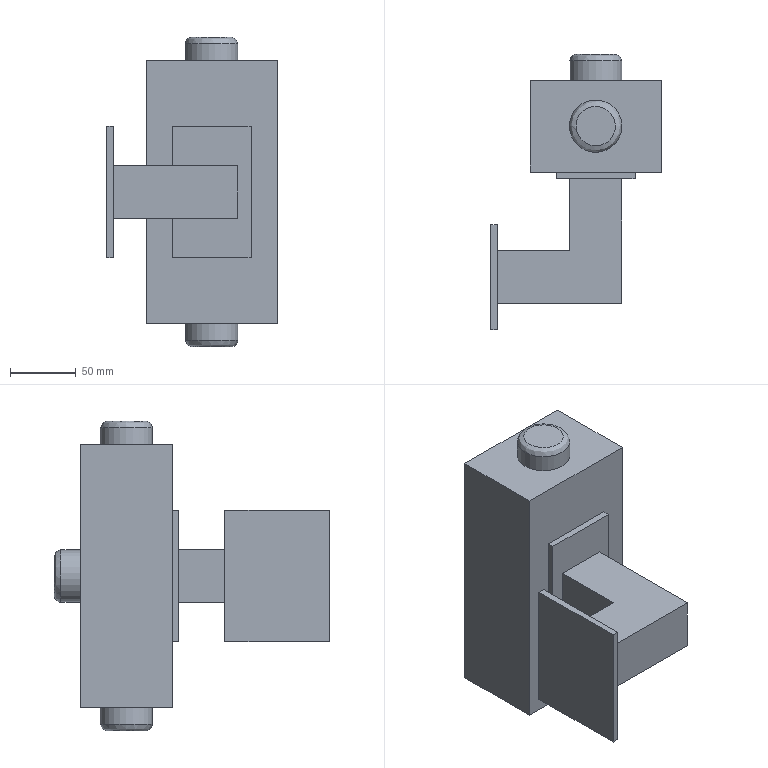Part | NX | features push bottom 6 | 5 solids | 44 faces | box 130 x 210 x 236 mm | volume 1605041 mm3 | plane 38 | spline 3 | cylinder 3 | commonest cylinder face diameters 40 x3